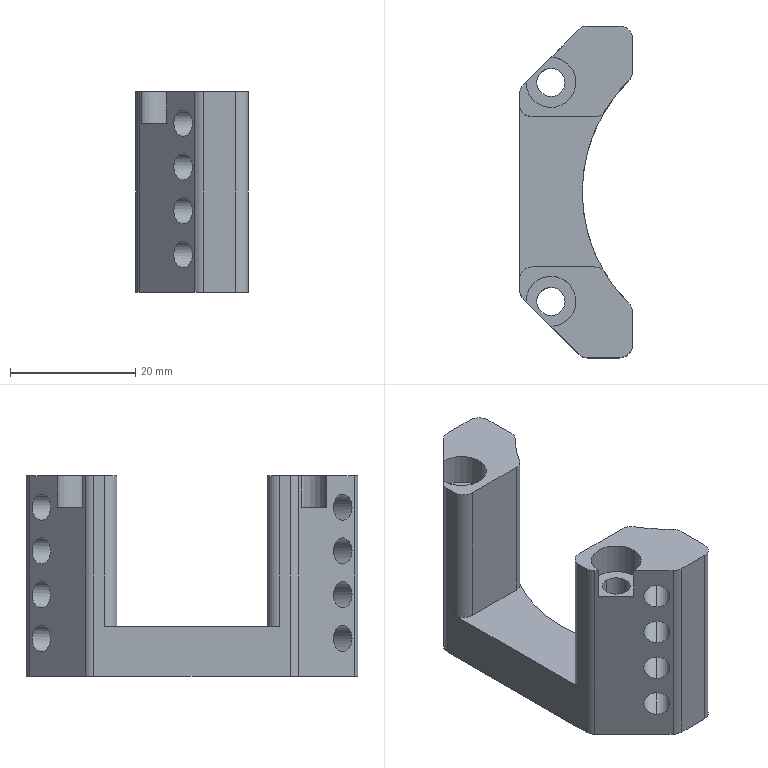NC program | Mastercam | posted with a generic post
Lines 12489 to 12929 of 15624:
N6100 T4 M6
N6110 G0 G90 G17 G54 X-16.37 Y3.6 A0. S6500 M3
N6120 G43 H4 Z50. M8
N6130 Z1.
N6140 G1 Z0. F600.
N6150 X-15.97 F2500.
N6160 G3 X-15.57 Y4. I0. J.4
N6170 X-17.5 Y5.93 Z-.075 I-1.93 J0.
N6180 X-19.43 Y4. Z-.15 I0. J-1.93
N6190 X-17.5 Y2.07 Z-.225 I1.93 J0.
N6200 X-15.57 Y4. Z-.3 I0. J1.93
N6210 X-17.5 Y5.93 Z-.375 I-1.93 J0.
N6220 X-19.43 Y4. Z-.45 I0. J-1.93
N6230 X-17.5 Y2.07 Z-.525 I1.93 J0.
N6240 X-15.57 Y4. Z-.6 I0. J1.93
N6250 X-17.5 Y5.93 Z-.675 I-1.93 J0.
N6260 X-19.43 Y4. Z-.75 I0. J-1.93
N6270 X-17.5 Y2.07 Z-.825 I1.93 J0.
N6280 X-15.57 Y4. Z-.9 I0. J1.93
N6290 X-17.5 Y5.93 Z-.975 I-1.93 J0.
N6300 X-19.43 Y4. Z-1.05 I0. J-1.93
N6310 X-17.5 Y2.07 Z-1.125 I1.93 J0.
N6320 X-15.57 Y4. Z-1.2 I0. J1.93
N6330 X-17.5 Y5.93 Z-1.275 I-1.93 J0.
N6340 X-19.43 Y4. Z-1.35 I0. J-1.93
N6350 X-17.5 Y2.07 Z-1.425 I1.93 J0.
N6360 X-15.57 Y4. Z-1.5 I0. J1.93
N6370 X-17.5 Y5.93 Z-1.575 I-1.93 J0.
N6380 X-19.43 Y4. Z-1.65 I0. J-1.93
N6390 X-17.5 Y2.07 Z-1.725 I1.93 J0.
N6400 X-15.57 Y4. Z-1.8 I0. J1.93
N6410 X-17.5 Y5.93 Z-1.875 I-1.93 J0.
N6420 X-19.43 Y4. Z-1.95 I0. J-1.93
N6430 X-17.5 Y2.07 Z-2.025 I1.93 J0.
N6440 X-15.57 Y4. Z-2.1 I0. J1.93
N6450 X-17.5 Y5.93 Z-2.175 I-1.93 J0.
N6460 X-19.43 Y4. Z-2.25 I0. J-1.93
N6470 X-17.5 Y2.07 Z-2.325 I1.93 J0.
N6480 X-15.57 Y4. Z-2.4 I0. J1.93
N6490 X-17.5 Y5.93 Z-2.475 I-1.93 J0.
N6500 X-19.43 Y4. Z-2.55 I0. J-1.93
N6510 X-17.5 Y2.07 Z-2.625 I1.93 J0.
N6520 X-15.57 Y4. Z-2.7 I0. J1.93
N6530 X-17.5 Y5.93 Z-2.775 I-1.93 J0.
N6540 X-19.43 Y4. Z-2.85 I0. J-1.93
N6550 X-17.5 Y2.07 Z-2.925 I1.93 J0.
N6560 X-15.57 Y4. Z-3. I0. J1.93
N6570 X-17.5 Y5.93 Z-3.075 I-1.93 J0.
N6580 X-19.43 Y4. Z-3.15 I0. J-1.93
N6590 X-17.5 Y2.07 Z-3.225 I1.93 J0.
N6600 X-15.57 Y4. Z-3.3 I0. J1.93
N6610 X-17.5 Y5.93 Z-3.375 I-1.93 J0.
N6620 X-19.43 Y4. Z-3.45 I0. J-1.93
N6630 X-17.5 Y2.07 Z-3.525 I1.93 J0.
N6640 X-15.57 Y4. Z-3.6 I0. J1.93
N6650 X-17.5 Y5.93 Z-3.675 I-1.93 J0.
N6660 X-19.43 Y4. Z-3.75 I0. J-1.93
N6670 X-17.5 Y2.07 Z-3.825 I1.93 J0.
N6680 X-15.57 Y4. Z-3.9 I0. J1.93
N6690 X-17.5 Y5.93 Z-3.975 I-1.93 J0.
N6700 X-19.43 Y4. Z-4.05 I0. J-1.93
N6710 X-17.5 Y2.07 Z-4.125 I1.93 J0.
N6720 X-15.57 Y4. Z-4.2 I0. J1.93
N6730 X-17.5 Y5.93 Z-4.275 I-1.93 J0.
N6740 X-19.43 Y4. Z-4.35 I0. J-1.93
N6750 X-17.5 Y2.07 Z-4.425 I1.93 J0.
N6760 X-15.57 Y4. Z-4.5 I0. J1.93
N6770 X-17.5 Y5.93 Z-4.575 I-1.93 J0.
N6780 X-19.43 Y4. Z-4.65 I0. J-1.93
N6790 X-17.5 Y2.07 Z-4.725 I1.93 J0.
N6800 X-15.57 Y4. Z-4.8 I0. J1.93
N6810 X-17.5 Y5.93 Z-4.875 I-1.93 J0.
N6820 X-19.43 Y4. Z-4.95 I0. J-1.93
N6830 X-17.5 Y2.07 I1.93 J0.
N6840 X-15.57 Y4. I0. J1.93
N6850 X-17.5 Y5.93 I-1.93 J0.
N6860 X-19.43 Y4. I0. J-1.93
N6870 X-19.03 Y3.6 I.4 J0.
N6880 G1 X-18.63
N6890 G0 Z50.
N6900 X18.63
N6910 Z1.
N6920 G1 Z0. F600.
N6930 X19.03 F2500.
N6940 G3 X19.43 Y4. I0. J.4
N6950 X17.5 Y5.93 Z-.075 I-1.93 J0.
N6960 X15.57 Y4. Z-.15 I0. J-1.93
N6970 X17.5 Y2.07 Z-.225 I1.93 J0.
N6980 X19.43 Y4. Z-.3 I0. J1.93
N6990 X17.5 Y5.93 Z-.375 I-1.93 J0.
N7000 X15.57 Y4. Z-.45 I0. J-1.93
N7010 X17.5 Y2.07 Z-.525 I1.93 J0.
N7020 X19.43 Y4. Z-.6 I0. J1.93
N7030 X17.5 Y5.93 Z-.675 I-1.93 J0.
N7040 X15.57 Y4. Z-.75 I0. J-1.93
N7050 X17.5 Y2.07 Z-.825 I1.93 J0.
N7060 X19.43 Y4. Z-.9 I0. J1.93
N7070 X17.5 Y5.93 Z-.975 I-1.93 J0.
N7080 X15.57 Y4. Z-1.05 I0. J-1.93
N7090 X17.5 Y2.07 Z-1.125 I1.93 J0.
N7100 X19.43 Y4. Z-1.2 I0. J1.93
N7110 X17.5 Y5.93 Z-1.275 I-1.93 J0.
N7120 X15.57 Y4. Z-1.35 I0. J-1.93
N7130 X17.5 Y2.07 Z-1.425 I1.93 J0.
N7140 X19.43 Y4. Z-1.5 I0. J1.93
N7150 X17.5 Y5.93 Z-1.575 I-1.93 J0.
N7160 X15.57 Y4. Z-1.65 I0. J-1.93
N7170 X17.5 Y2.07 Z-1.725 I1.93 J0.
N7180 X19.43 Y4. Z-1.8 I0. J1.93
N7190 X17.5 Y5.93 Z-1.875 I-1.93 J0.
N7200 X15.57 Y4. Z-1.95 I0. J-1.93
N7210 X17.5 Y2.07 Z-2.025 I1.93 J0.
N7220 X19.43 Y4. Z-2.1 I0. J1.93
N7230 X17.5 Y5.93 Z-2.175 I-1.93 J0.
N7240 X15.57 Y4. Z-2.25 I0. J-1.93
N7250 X17.5 Y2.07 Z-2.325 I1.93 J0.
N7260 X19.43 Y4. Z-2.4 I0. J1.93
N7270 X17.5 Y5.93 Z-2.475 I-1.93 J0.
N7280 X15.57 Y4. Z-2.55 I0. J-1.93
N7290 X17.5 Y2.07 Z-2.625 I1.93 J0.
N7300 X19.43 Y4. Z-2.7 I0. J1.93
N7310 X17.5 Y5.93 Z-2.775 I-1.93 J0.
N7320 X15.57 Y4. Z-2.85 I0. J-1.93
N7330 X17.5 Y2.07 Z-2.925 I1.93 J0.
N7340 X19.43 Y4. Z-3. I0. J1.93
N7350 X17.5 Y5.93 Z-3.075 I-1.93 J0.
N7360 X15.57 Y4. Z-3.15 I0. J-1.93
N7370 X17.5 Y2.07 Z-3.225 I1.93 J0.
N7380 X19.43 Y4. Z-3.3 I0. J1.93
N7390 X17.5 Y5.93 Z-3.375 I-1.93 J0.
N7400 X15.57 Y4. Z-3.45 I0. J-1.93
N7410 X17.5 Y2.07 Z-3.525 I1.93 J0.
N7420 X19.43 Y4. Z-3.6 I0. J1.93
N7430 X17.5 Y5.93 Z-3.675 I-1.93 J0.
N7440 X15.57 Y4. Z-3.75 I0. J-1.93
N7450 X17.5 Y2.07 Z-3.825 I1.93 J0.
N7460 X19.43 Y4. Z-3.9 I0. J1.93
N7470 X17.5 Y5.93 Z-3.975 I-1.93 J0.
N7480 X15.57 Y4. Z-4.05 I0. J-1.93
N7490 X17.5 Y2.07 Z-4.125 I1.93 J0.
N7500 X19.43 Y4. Z-4.2 I0. J1.93
N7510 X17.5 Y5.93 Z-4.275 I-1.93 J0.
N7520 X15.57 Y4. Z-4.35 I0. J-1.93
N7530 X17.5 Y2.07 Z-4.425 I1.93 J0.
N7540 X19.43 Y4. Z-4.5 I0. J1.93
N7550 X17.5 Y5.93 Z-4.575 I-1.93 J0.
N7560 X15.57 Y4. Z-4.65 I0. J-1.93
N7570 X17.5 Y2.07 Z-4.725 I1.93 J0.
N7580 X19.43 Y4. Z-4.8 I0. J1.93
N7590 X17.5 Y5.93 Z-4.875 I-1.93 J0.
N7600 X15.57 Y4. Z-4.95 I0. J-1.93
N7610 X17.5 Y2.07 I1.93 J0.
N7620 X19.43 Y4. I0. J1.93
N7630 X17.5 Y5.93 I-1.93 J0.
N7640 X15.57 Y4. I0. J-1.93
N7650 X15.97 Y3.6 I.4 J0.
N7660 G1 X16.37
N7670 G0 Z50.
N7680 X-16.29
N7690 Z1.
N7700 G1 Z-5. F600.
N7710 X-15.89 F1000.
N7720 G3 X-15.49 Y4. I0. J.4
N7730 X-17.5 Y6.01 I-2.01 J0.
N7740 X-19.51 Y4. I0. J-2.01
N7750 X-17.5 Y1.99 I2.01 J0.
N7760 X-15.49 Y4. I0. J2.01
N7770 X-15.89 Y4.4 I-.4 J0.
N7780 G1 X-16.29
N7790 G0 Z50.
N7800 X18.71 Y3.6
N7810 Z1.
N7820 G1 Z-5. F600.
N7830 X19.11 F1000.
N7840 G3 X19.51 Y4. I0. J.4
N7850 X17.5 Y6.01 I-2.01 J0.
N7860 X15.49 Y4. I0. J-2.01
N7870 X17.5 Y1.99 I2.01 J0.
N7880 X19.51 Y4. I0. J2.01
N7890 X19.11 Y4.4 I-.4 J0.
N7900 G1 X18.71
N7910 G0 Z50.
N7920 M5
N7930 G91 G28 Z0. M9
N7940 A0.
N7950 M01
N7960 T12 M6
N7970 G0 G90 G17 G54 X-2.164 Y15. A0. S6000 M3
N7980 G43 H12 Z50. M8
N7990 Z-23.
N8000 G1 Z-24. F600.
N8010 Y14.162 F1000.
N8020 G2 X.022 Y4.946 I-18.331 J-9.216
N8030 X-.164 Y2.189 I-20.517 J0.
N8040 G1 X-.429 Y-5.505
N8050 X-.011 Y-7.001
N8060 G3 X.545 Y-7.422 I.556 J.156
N8070 X.915 Y-7.289 I0. J.577
N8080 X1.123 Y-6.845 I-.37 J.444
N8090 X.797 Y-6.326 I-.578 J0.
N8100 G1 X-.598 Y-5.651
N8110 G3 X-1.101 Y-5.536 I-.503 J-1.039
N8120 X-2.255 Y-6.69 I0. J-1.154
N8130 X-2.154 Y-7.165 I1.154 J0.
N8140 X-1.101 Y-7.845 I1.053 J.475
N8150 X.011 Y-7.001 I0. J1.155
N8160 G1 X.429 Y-5.505
N8170 G2 X.023 Y2.459 I77.922 J7.964
N8180 X.245 Y8.352 I78.328 J0.
N8190 X2.164 Y14.162 I18.475 J-2.882
N8200 G1 Y15.
N8210 G3 X1.009 Y16.155 I-1.155 J0.
N8220 G1 X-6.645
N8230 G3 X-7.8 Y15. I0. J-1.155
N8240 G1 Y12.335
N8250 X-7.799 Y12.332
N8260 X-7.712 Y12.23
N8270 X-7.118 Y11.458
N8280 X-6.949 Y11.184
N8290 G2 X-6.085 Y9.141 I-9.337 J-5.154
N8300 G1 X-5.934 Y8.368
N8310 X-5.83 Y7.596
N8320 X-5.8 Y6.824
N8330 Y2.189
N8340 X-5.808 Y-3.218
N8350 X-6.017 Y-4.762
N8360 X-6.254 Y-5.598
N8370 X-5.62 Y-7.872
N8380 X-5.545 Y-8.036
N8390 X-5.423 Y-8.169
N8400 X-5.266 Y-8.258
N8410 X-5.089 Y-8.293
N8420 X4.456 Y-8.715
N8430 G3 X4.507 Y-8.716 I.051 J1.154
N8440 X5.62 Y-7.872 I0. J1.155
N8450 G1 X6.254 Y-5.598
N8460 X6.017 Y-4.762
N8470 X5.808 Y-3.218
N8480 G2 X5.782 Y2.24 I567.892 J5.458
N8490 X5.8 Y6.824 I567.918 J0.
N8500 G1 X5.83 Y7.596
N8510 G2 X6.346 Y9.913 I8.398 J-.654
N8520 G1 X6.949 Y11.184
N8530 X7.118 Y11.458
N8540 X7.8 Y12.335
N8550 Y15.
N8560 G0 Z50.
N8570 X-30.425 Y-15.631
N8580 Z1.
N8590 G1 Z-12. F600.
N8600 X-29.637 Y-14.726 F1000.
N8610 G3 X-29.342 Y-13.938 I-.905 J.788
N8620 X-29.754 Y-13.033 I-1.2 J0.
N8630 G2 X-32.5 Y-7. I5.254 J6.033
N8640 G1 Y-1.828
N8650 G2 X-30.157 Y3.828 I8. J0.
N8660 G1 X-25.743 Y8.243
N8670 X-21.743 Y12.243
N8680 X-21.328 Y12.657
N8690 G2 X-15.672 Y15. I5.656 J-5.657
N8700 G1 X-14.
N8710 G2 X-6. Y7. I0. J-8.
N8720 G1 Y-2.913
N8730 G2 X-9.852 Y-9.754 I-8. J0.
N8740 G3 X-13.499 Y-12.63 I9.852 J-16.246
N8750 G2 X-19.183 Y-15. I-5.684 J5.63
N8760 G1 X-24.5
N8770 G2 X-29.754 Y-13.033 I0. J8.
N8780 G3 X-30.542 Y-12.738 I-.788 J-.905
N8790 X-31.447 Y-13.15 I0. J-1.2
N8800 G1 X-32.235 Y-14.054
N8810 X-30.425 Y-15.631
N8820 Z-24. F600.
N8830 X-29.637 Y-14.726 F1000.
N8840 G3 X-29.342 Y-13.938 I-.905 J.788
N8850 X-29.754 Y-13.033 I-1.2 J0.
N8860 G2 X-32.5 Y-7. I5.254 J6.033
N8870 G1 Y-1.828
N8880 G2 X-30.157 Y3.828 I8. J0.
N8890 G1 X-25.743 Y8.243
N8900 X-21.743 Y12.243
N8910 X-21.328 Y12.657
N8920 G2 X-15.672 Y15. I5.656 J-5.657
N8930 G1 X-14.
N8940 G2 X-6. Y7. I0. J-8.
N8950 G1 Y-2.913
N8960 G2 X-9.852 Y-9.754 I-8. J0.
N8970 G3 X-13.499 Y-12.63 I9.852 J-16.246
N8980 G2 X-19.183 Y-15. I-5.684 J5.63
N8990 G1 X-24.5
N9000 G2 X-29.754 Y-13.033 I0. J8.
N9010 G3 X-30.542 Y-12.738 I-.788 J-.905
N9020 X-31.447 Y-13.15 I0. J-1.2
N9030 G1 X-32.235 Y-14.054
N9040 G0 Z50.
N9050 X32.624 Y-13.603
N9060 Z1.
N9070 G1 Z-12. F600.
N9080 X31.786 Y-12.744 F1000.
N9090 G3 X30.927 Y-12.382 I-.859 J-.838
N9100 X30.089 Y-12.724 I0. J-1.2
N9110 G2 X24.5 Y-15. I-5.589 J5.724
N9120 G1 X19.183
N9130 G2 X13.499 Y-12.63 I0. J8.
N9140 G3 X9.852 Y-9.754 I-13.499 J-13.37
N9150 G2 X6. Y-2.913 I4.148 J6.841
N9160 G1 Y7.
N9170 G2 X14. Y15. I8. J0.
N9180 G1 X15.672
N9190 G2 X21.328 Y12.657 I0. J-8.
N9200 G1 X21.743 Y12.243
N9210 X25.743 Y8.243
N9220 X30.157 Y3.828
N9230 G2 X32.5 Y-1.828 I-5.657 J-5.656
N9240 G1 Y-7.
N9250 G2 X30.089 Y-12.724 I-8. J0.
N9260 G3 X29.728 Y-13.582 I.838 J-.858
N9270 X30.069 Y-14.421 I1.199 J0.
N9280 G1 X30.907 Y-15.279
N9290 X32.624 Y-13.603
N9300 Z-24. F600.
N9310 X31.786 Y-12.744 F1000.
N9320 G3 X30.927 Y-12.382 I-.859 J-.838
N9330 X30.089 Y-12.724 I0. J-1.2
N9340 G2 X24.5 Y-15. I-5.589 J5.724
N9350 G1 X19.183
N9360 G2 X13.499 Y-12.63 I0. J8.
N9370 G3 X9.852 Y-9.754 I-13.499 J-13.37
N9380 G2 X6. Y-2.913 I4.148 J6.841
N9390 G1 Y7.
N9400 G2 X14. Y15. I8. J0.
N9410 G1 X15.672
N9420 G2 X21.328 Y12.657 I0. J-8.
N9430 G1 X21.743 Y12.243
N9440 X25.743 Y8.243
N9450 X30.157 Y3.828
N9460 G2 X32.5 Y-1.828 I-5.657 J-5.656
N9470 G1 Y-7.
N9480 G2 X30.089 Y-12.724 I-8. J0.
N9490 G3 X29.728 Y-13.582 I.838 J-.858
N9500 X30.069 Y-14.421 I1.199 J0.
N9510 G1 X30.907 Y-15.279
N9520 G0 Z50.
N9530 X31.5 Y-14.785
N9540 Z-31.
N9550 G1 Z-32.5 F600.
N9560 X30.805 Y-13.807 F1000.
N9570 G3 X29.826 Y-13.301 I-.979 J-.694
N9580 X29.132 Y-13.523 I0. J-1.2
N9590 G2 X24.5 Y-15. I-4.632 J6.523
N9600 G1 X19.183
N9610 G2 X13.499 Y-12.63 I0. J8.
N9620 G3 X0. Y-7.001 I-13.499 J-13.37
N9630 X-13.499 Y-12.63 I0. J-18.999
N9640 G2 X-19.183 Y-15. I-5.684 J5.63
N9650 G1 X-24.5
N9660 G2 X-32.5 Y-7. I0. J8.
N9670 G1 Y-1.828
N9680 G2 X-30.157 Y3.828 I8. J0.
N9690 G1 X-21.328 Y12.657
N9700 G2 X-15.672 Y15. I5.656 J-5.657
N9710 G1 X15.672
N9720 G2 X21.328 Y12.657 I0. J-8.
N9730 G1 X30.157 Y3.828
N9740 G2 X32.5 Y-1.828 I-5.657 J-5.656
N9750 G1 Y-7.
N9760 G2 X29.132 Y-13.523 I-8. J0.
N9770 G3 X28.627 Y-14.501 I.694 J-.978
N9780 X28.848 Y-15.196 I1.199 J0.
N9790 G1 X29.543 Y-16.174
N9800 G0 Z50.
N9810 M5
N9820 G91 G28 Z0. M9
N9830 A0.
N9840 M01
N9850 T5 M6
N9860 G0 G90 G17 G54 X-17.5 Y4. A0. S6000 M3
N9870 G43 H5 Z45. M8
N9880 G98 G81 Z-5.7 R-4. F200.
N9890 X17.5
N9900 G80
N9910 G0 X-18.783 Y-10.45 Z50.
N9920 Z1.
N9930 G1 Z-.75 F600.
N9940 Y-10.05 F1000.
N9950 G3 X-19.183 Y-9.65 I-.4 J0.
N9960 G1 X-24.5
N9970 G2 X-27.15 Y-7. I0. J2.65
N9980 G1 Y-1.828
N9990 G2 X-26.374 Y.045 I2.65 J0.
N100 G1 X-21.96 Y4.46
N110 G2 X-21.5 Y4.651 I.46 J-.46
N120 X-20.85 Y4. I0. J-.651
N130 G3 X-17.5 Y.65 I3.35 J0.
N140 X-14.15 Y4. I0. J3.35
N150 X-17.5 Y7.35 I-3.35 J0.
N160 G2 X-18.15 Y8. I0. J.65
N170 X-17.96 Y8.46 I.65 J0.
N180 G1 X-17.545 Y8.874
N190 G2 X-15.672 Y9.65 I1.873 J-1.874
N200 G1 X-14.
N210 G2 X-11.35 Y7. I0. J-2.65
N220 G1 Y-2.913
N230 G2 X-12.626 Y-5.179 I-2.65 J0.
N240 G3 X-17.301 Y-8.865 I12.626 J-20.821
N250 G2 X-19.183 Y-9.65 I-1.882 J1.865
N260 G3 X-19.583 Y-10.05 I0. J-.4
N270 G1 Y-10.45
N280 G0 Z50.
N290 X24.9
N300 Z1.
N310 G1 Z-.75 F600.
N320 Y-10.05 F1000.
N330 G3 X24.5 Y-9.65 I-.4 J0.
N340 G1 X19.183
N350 G2 X17.301 Y-8.865 I0. J2.65
N360 G3 X12.626 Y-5.179 I-17.301 J-17.135
N370 G2 X11.35 Y-2.913 I1.374 J2.266
N380 G1 Y7.
N390 G2 X14. Y9.65 I2.65 J0.
N400 G1 X15.672
N410 G2 X17.545 Y8.874 I0. J-2.65
N420 G1 X17.96 Y8.46
N430 G2 X18.151 Y8. I-.46 J-.46
N440 X17.5 Y7.35 I-.651 J0.
N450 G3 X14.15 Y4. I0. J-3.35
N460 X17.5 Y.65 I3.35 J0.
N470 X20.85 Y4. I0. J3.35
N480 G2 X21.5 Y4.65 I.65 J0.
N490 X21.96 Y4.46 I0. J-.65
N500 G1 X26.374 Y.045
N510 G2 X27.15 Y-1.828 I-1.874 J-1.873
N520 G1 Y-7.
N530 G2 X24.5 Y-9.65 I-2.65 J0.
N540 G3 X24.1 Y-10.05 I0. J-.4
N550 G1 Y-10.45
N560 G0 Z50.
N570 M5
N580 G91 G28 Z0. M9
N590 A0.
N600 M01